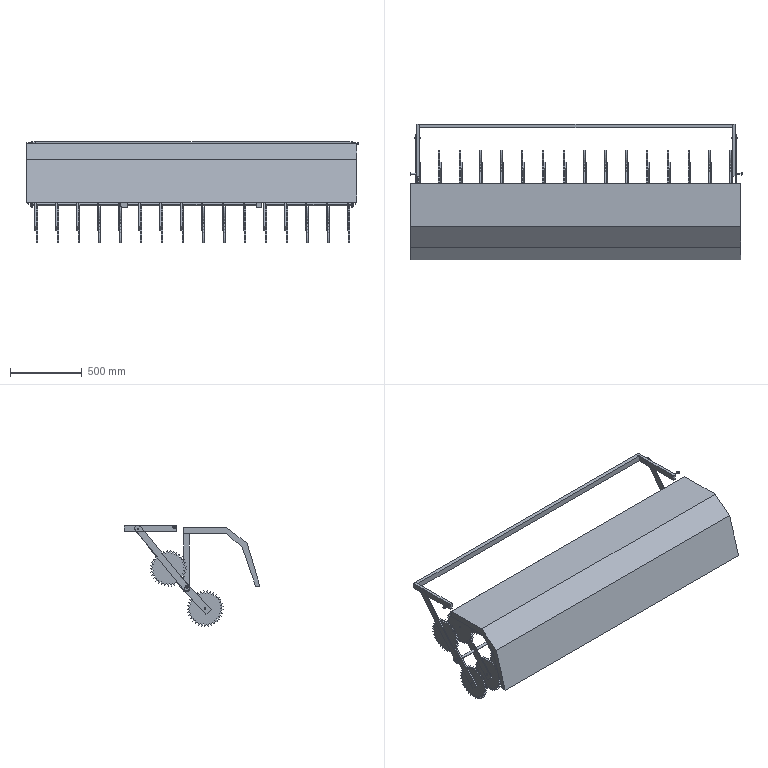Part | SolidWorks | features ReferencePattern 16, CompositeCurve 3, LocalLPattern 1, MirrorCompFeat 1 | 61 solids | 2653 faces | box 2314 x 946.381 x 704.175 mm | volume 91068773 mm3 | plane 2371 | cylinder 246 | cone 28 | sphere 4 | torus 4 | commonest cylinder face diameters 10 x140 20 x42 1.79 x16 8 x12 3.132 x8 3.133 x6